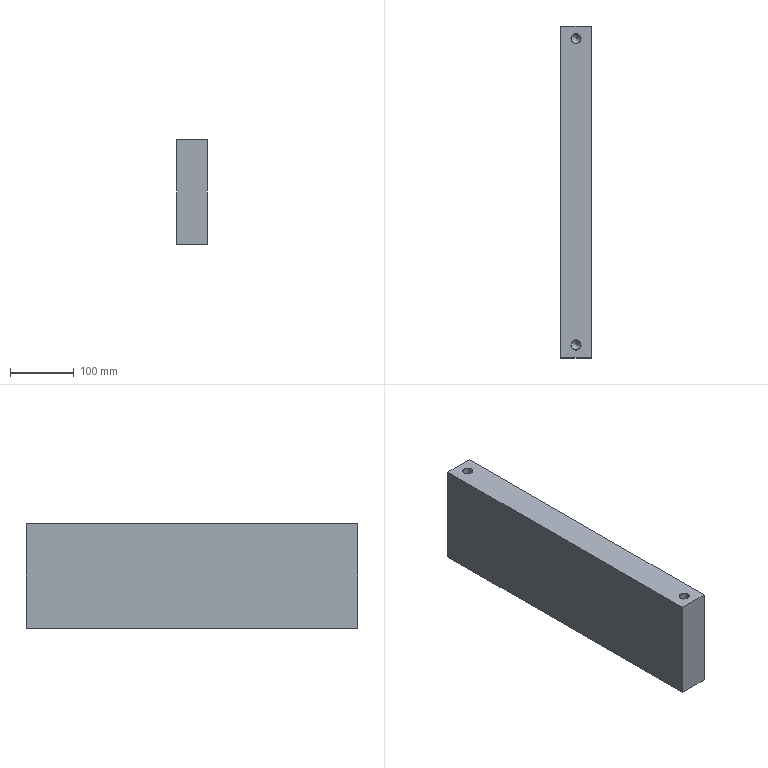Part | NX | features B2-3 2 | 1 solid | 18 faces | box 48 x 520 x 163 mm | volume 4027167 mm3 | cone 8 | plane 6 | cylinder 4 | commonest cylinder face diameters 14.506 x4
STEP:
#1=CARTESIAN_POINT('',(3450.094,-599.122,733.716));
#2=VERTEX_POINT('',#1);
#3=CARTESIAN_POINT('',(3450.094,-1119.122,733.716));
#4=VERTEX_POINT('',#3);
#5=CARTESIAN_POINT('',(3450.094,-599.122,733.716));
#6=DIRECTION('',(0.,-1.,0.));
#7=VECTOR('',#6,1000.);
#8=LINE('',#5,#7);
#9=EDGE_CURVE('',#2,#4,#8,.T.);
#10=ORIENTED_EDGE('',*,*,#9,.T.);
#11=CARTESIAN_POINT('',(3450.094,-1119.122,570.716));
#12=VERTEX_POINT('',#11);
#13=CARTESIAN_POINT('',(3450.094,-1119.122,600.716));
#14=DIRECTION('',(0.,0.,1.));
#15=VECTOR('',#14,1000.);
#16=LINE('',#13,#15);
#17=EDGE_CURVE('',#12,#4,#16,.T.);
#18=ORIENTED_EDGE('',*,*,#17,.F.);
#19=CARTESIAN_POINT('',(3450.094,-599.122,570.716));
#20=VERTEX_POINT('',#19);
#21=CARTESIAN_POINT('',(3450.094,-599.122,570.716));
#22=DIRECTION('',(0.,-1.,0.));
#23=VECTOR('',#22,1000.);
#24=LINE('',#21,#23);
#25=EDGE_CURVE('',#20,#12,#24,.T.);
#26=ORIENTED_EDGE('',*,*,#25,.F.);
#27=CARTESIAN_POINT('',(3450.094,-599.122,600.716));
#28=DIRECTION('',(0.,0.,1.));
#29=VECTOR('',#28,1000.);
#30=LINE('',#27,#29);
#31=EDGE_CURVE('',#20,#2,#30,.T.);
#32=ORIENTED_EDGE('',*,*,#31,.T.);
#33=EDGE_LOOP('',(#10,#18,#26,#32));
#34=FACE_BOUND('',#33,.T.);
#35=CARTESIAN_POINT('',(3450.094,-599.122,600.716));
#36=DIRECTION('',(-1.,0.,0.));
#37=DIRECTION('',(0.,0.,1.));
#38=AXIS2_PLACEMENT_3D('',#35,#36,#37);
#39=PLANE('',#38);
#40=ADVANCED_FACE('',(#34),#39,.F.);
#41=CARTESIAN_POINT('',(3418.094,-1039.122,570.716));
#42=VERTEX_POINT('',#41);
#43=CARTESIAN_POINT('',(3426.094,-1039.122,570.716));
#44=DIRECTION('',(0.,0.,-1.));
#45=DIRECTION('',(-1.,0.,0.));
#46=AXIS2_PLACEMENT_3D('',#43,#44,#45);
#47=CIRCLE('',#46,8.);
#48=EDGE_CURVE('',#42,#42,#47,.T.);
#49=ORIENTED_EDGE('',*,*,#48,.F.);
#50=EDGE_LOOP('',(#49));
#51=FACE_BOUND('',#50,.T.);
#52=CARTESIAN_POINT('',(3418.094,-679.122,570.716));
#53=VERTEX_POINT('',#52);
#54=CARTESIAN_POINT('',(3426.094,-679.122,570.716));
#55=DIRECTION('',(0.,0.,-1.));
#56=DIRECTION('',(-1.,0.,0.));
#57=AXIS2_PLACEMENT_3D('',#54,#55,#56);
#58=CIRCLE('',#57,8.);
#59=EDGE_CURVE('',#53,#53,#58,.T.);
#60=ORIENTED_EDGE('',*,*,#59,.F.);
#61=EDGE_LOOP('',(#60));
#62=FACE_BOUND('',#61,.T.);
#63=CARTESIAN_POINT('',(3402.094,-599.122,570.716));
#64=VERTEX_POINT('',#63);
#65=CARTESIAN_POINT('',(3402.094,-1119.122,570.716));
#66=VERTEX_POINT('',#65);
#67=CARTESIAN_POINT('',(3402.094,0.,570.716));
#68=DIRECTION('',(0.,-1.,0.));
#69=VECTOR('',#68,1000.);
#70=LINE('',#67,#69);
#71=EDGE_CURVE('',#64,#66,#70,.T.);
#72=ORIENTED_EDGE('',*,*,#71,.F.);
#73=CARTESIAN_POINT('',(1325.094,-599.122,570.716));
#74=DIRECTION('',(1.,0.,0.));
#75=VECTOR('',#74,1000.);
#76=LINE('',#73,#75);
#77=EDGE_CURVE('',#64,#20,#76,.T.);
#78=ORIENTED_EDGE('',*,*,#77,.T.);
#79=ORIENTED_EDGE('',*,*,#25,.T.);
#80=CARTESIAN_POINT('',(3450.094,-1119.122,570.716));
#81=DIRECTION('',(-1.,0.,0.));
#82=VECTOR('',#81,1000.);
#83=LINE('',#80,#82);
#84=EDGE_CURVE('',#12,#66,#83,.T.);
#85=ORIENTED_EDGE('',*,*,#84,.T.);
#86=EDGE_LOOP('',(#72,#78,#79,#85));
#87=FACE_BOUND('',#86,.T.);
#88=CARTESIAN_POINT('',(-930.,0.,570.716));
#89=DIRECTION('',(0.,0.,-1.));
#90=DIRECTION('',(-1.,0.,0.));
#91=AXIS2_PLACEMENT_3D('',#88,#89,#90);
#92=PLANE('',#91);
#93=ADVANCED_FACE('',(#51,#62,#87),#92,.T.);
#94=CARTESIAN_POINT('',(3434.094,-619.122,733.716));
#95=VERTEX_POINT('',#94);
#96=CARTESIAN_POINT('',(3426.094,-619.122,733.716));
#97=DIRECTION('',(0.,0.,1.));
#98=DIRECTION('',(1.,0.,0.));
#99=AXIS2_PLACEMENT_3D('',#96,#97,#98);
#100=CIRCLE('',#99,8.);
#101=EDGE_CURVE('',#95,#95,#100,.T.);
#102=ORIENTED_EDGE('',*,*,#101,.F.);
#103=EDGE_LOOP('',(#102));
#104=FACE_BOUND('',#103,.T.);
#105=CARTESIAN_POINT('',(3434.094,-1099.122,733.716));
#106=VERTEX_POINT('',#105);
#107=CARTESIAN_POINT('',(3426.094,-1099.122,733.716));
#108=DIRECTION('',(0.,0.,1.));
#109=DIRECTION('',(1.,0.,0.));
#110=AXIS2_PLACEMENT_3D('',#107,#108,#109);
#111=CIRCLE('',#110,8.);
#112=EDGE_CURVE('',#106,#106,#111,.T.);
#113=ORIENTED_EDGE('',*,*,#112,.F.);
#114=EDGE_LOOP('',(#113));
#115=FACE_BOUND('',#114,.T.);
#116=CARTESIAN_POINT('',(3402.094,-599.122,733.716));
#117=VERTEX_POINT('',#116);
#118=CARTESIAN_POINT('',(1325.094,-599.122,733.716));
#119=DIRECTION('',(1.,0.,0.));
#120=VECTOR('',#119,1000.);
#121=LINE('',#118,#120);
#122=EDGE_CURVE('',#117,#2,#121,.T.);
#123=ORIENTED_EDGE('',*,*,#122,.F.);
#124=CARTESIAN_POINT('',(3402.094,-1119.122,733.716));
#125=VERTEX_POINT('',#124);
#126=CARTESIAN_POINT('',(3402.094,-859.122,733.716));
#127=DIRECTION('',(0.,1.,0.));
#128=VECTOR('',#127,1000.);
#129=LINE('',#126,#128);
#130=EDGE_CURVE('',#125,#117,#129,.T.);
#131=ORIENTED_EDGE('',*,*,#130,.F.);
#132=CARTESIAN_POINT('',(3450.094,-1119.122,733.716));
#133=DIRECTION('',(-1.,0.,0.));
#134=VECTOR('',#133,1000.);
#135=LINE('',#132,#134);
#136=EDGE_CURVE('',#4,#125,#135,.T.);
#137=ORIENTED_EDGE('',*,*,#136,.F.);
#138=ORIENTED_EDGE('',*,*,#9,.F.);
#139=EDGE_LOOP('',(#123,#131,#137,#138));
#140=FACE_BOUND('',#139,.T.);
#141=CARTESIAN_POINT('',(-930.,0.,733.716));
#142=DIRECTION('',(0.,0.,-1.));
#143=DIRECTION('',(-1.,0.,0.));
#144=AXIS2_PLACEMENT_3D('',#141,#142,#143);
#145=PLANE('',#144);
#146=ADVANCED_FACE('',(#104,#115,#140),#145,.F.);
#147=ORIENTED_EDGE('',*,*,#136,.T.);
#148=CARTESIAN_POINT('',(3402.094,-1119.122,600.716));
#149=DIRECTION('',(0.,0.,-1.));
#150=VECTOR('',#149,1000.);
#151=LINE('',#148,#150);
#152=EDGE_CURVE('',#125,#66,#151,.T.);
#153=ORIENTED_EDGE('',*,*,#152,.T.);
#154=ORIENTED_EDGE('',*,*,#84,.F.);
#155=ORIENTED_EDGE('',*,*,#17,.T.);
#156=EDGE_LOOP('',(#147,#153,#154,#155));
#157=FACE_BOUND('',#156,.T.);
#158=CARTESIAN_POINT('',(3450.094,-1119.122,600.716));
#159=DIRECTION('',(0.,1.,0.));
#160=DIRECTION('',(-1.,0.,0.));
#161=AXIS2_PLACEMENT_3D('',#158,#159,#160);
#162=PLANE('',#161);
#163=ADVANCED_FACE('',(#157),#162,.F.);
#164=ORIENTED_EDGE('',*,*,#77,.F.);
#165=CARTESIAN_POINT('',(3402.094,-599.122,600.716));
#166=DIRECTION('',(0.,0.,1.));
#167=VECTOR('',#166,1000.);
#168=LINE('',#165,#167);
#169=EDGE_CURVE('',#64,#117,#168,.T.);
#170=ORIENTED_EDGE('',*,*,#169,.T.);
#171=ORIENTED_EDGE('',*,*,#122,.T.);
#172=ORIENTED_EDGE('',*,*,#31,.F.);
#173=EDGE_LOOP('',(#164,#170,#171,#172));
#174=FACE_BOUND('',#173,.T.);
#175=CARTESIAN_POINT('',(1325.094,-599.122,600.716));
#176=DIRECTION('',(0.,-1.,0.));
#177=DIRECTION('',(0.,0.,-1.));
#178=AXIS2_PLACEMENT_3D('',#175,#176,#177);
#179=PLANE('',#178);
#180=ADVANCED_FACE('',(#174),#179,.F.);
#181=ORIENTED_EDGE('',*,*,#71,.T.);
#182=ORIENTED_EDGE('',*,*,#152,.F.);
#183=ORIENTED_EDGE('',*,*,#130,.T.);
#184=ORIENTED_EDGE('',*,*,#169,.F.);
#185=EDGE_LOOP('',(#181,#182,#183,#184));
#186=FACE_BOUND('',#185,.T.);
#187=CARTESIAN_POINT('',(3402.094,-859.122,667.216));
#188=DIRECTION('',(1.,0.,0.));
#189=DIRECTION('',(0.,0.,-1.));
#190=AXIS2_PLACEMENT_3D('',#187,#188,#189);
#191=PLANE('',#190);
#192=ADVANCED_FACE('',(#186),#191,.F.);
#193=CARTESIAN_POINT('',(3433.347,-1099.122,732.969));
#194=VERTEX_POINT('',#193);
#195=CARTESIAN_POINT('',(3426.094,-1099.122,732.969));
#196=DIRECTION('',(0.,0.,1.));
#197=DIRECTION('',(1.,0.,0.));
#198=AXIS2_PLACEMENT_3D('',#195,#196,#197);
#199=CIRCLE('',#198,7.253);
#200=EDGE_CURVE('',#194,#194,#199,.F.);
#201=ORIENTED_EDGE('',*,*,#200,.F.);
#202=EDGE_LOOP('',(#201));
#203=FACE_BOUND('',#202,.T.);
#204=CARTESIAN_POINT('',(3433.347,-1099.122,688.719));
#205=VERTEX_POINT('',#204);
#206=CARTESIAN_POINT('',(3426.094,-1099.122,688.719));
#207=DIRECTION('',(0.,0.,1.));
#208=DIRECTION('',(1.,0.,0.));
#209=AXIS2_PLACEMENT_3D('',#206,#207,#208);
#210=CIRCLE('',#209,7.253);
#211=EDGE_CURVE('',#205,#205,#210,.F.);
#212=ORIENTED_EDGE('',*,*,#211,.T.);
#213=EDGE_LOOP('',(#212));
#214=FACE_BOUND('',#213,.T.);
#215=CARTESIAN_POINT('',(3426.094,-1099.122,681.466));
#216=DIRECTION('',(0.,0.,1.));
#217=DIRECTION('',(1.,0.,0.));
#218=AXIS2_PLACEMENT_3D('',#215,#216,#217);
#219=CYLINDRICAL_SURFACE('',#218,7.253);
#220=ADVANCED_FACE('',(#203,#214),#219,.F.);
#221=CARTESIAN_POINT('',(3426.094,-1099.122,681.466));
#222=VERTEX_POINT('',#221);
#223=VERTEX_LOOP('',#222);
#224=FACE_BOUND('',#223,.T.);
#225=ORIENTED_EDGE('',*,*,#211,.F.);
#226=EDGE_LOOP('',(#225));
#227=FACE_BOUND('',#226,.T.);
#228=CARTESIAN_POINT('',(3426.094,-1099.122,688.716));
#229=DIRECTION('',(0.,0.,1.));
#230=DIRECTION('',(1.,0.,0.));
#231=AXIS2_PLACEMENT_3D('',#228,#229,#230);
#232=CONICAL_SURFACE('',#231,7.25,0.7854);
#233=ADVANCED_FACE('',(#224,#227),#232,.F.);
#234=ORIENTED_EDGE('',*,*,#200,.T.);
#235=EDGE_LOOP('',(#234));
#236=FACE_BOUND('',#235,.T.);
#237=ORIENTED_EDGE('',*,*,#112,.T.);
#238=EDGE_LOOP('',(#237));
#239=FACE_BOUND('',#238,.T.);
#240=CARTESIAN_POINT('',(3426.094,-1099.122,733.716));
#241=DIRECTION('',(0.,0.,1.));
#242=DIRECTION('',(1.,0.,0.));
#243=AXIS2_PLACEMENT_3D('',#240,#241,#242);
#244=CONICAL_SURFACE('',#243,8.,0.7854);
#245=ADVANCED_FACE('',(#236,#239),#244,.F.);
#246=CARTESIAN_POINT('',(3433.347,-619.122,732.969));
#247=VERTEX_POINT('',#246);
#248=CARTESIAN_POINT('',(3426.094,-619.122,732.969));
#249=DIRECTION('',(0.,0.,1.));
#250=DIRECTION('',(1.,0.,0.));
#251=AXIS2_PLACEMENT_3D('',#248,#249,#250);
#252=CIRCLE('',#251,7.253);
#253=EDGE_CURVE('',#247,#247,#252,.F.);
#254=ORIENTED_EDGE('',*,*,#253,.F.);
#255=EDGE_LOOP('',(#254));
#256=FACE_BOUND('',#255,.T.);
#257=CARTESIAN_POINT('',(3433.347,-619.122,688.719));
#258=VERTEX_POINT('',#257);
#259=CARTESIAN_POINT('',(3426.094,-619.122,688.719));
#260=DIRECTION('',(0.,0.,1.));
#261=DIRECTION('',(1.,0.,0.));
#262=AXIS2_PLACEMENT_3D('',#259,#260,#261);
#263=CIRCLE('',#262,7.253);
#264=EDGE_CURVE('',#258,#258,#263,.F.);
#265=ORIENTED_EDGE('',*,*,#264,.T.);
#266=EDGE_LOOP('',(#265));
#267=FACE_BOUND('',#266,.T.);
#268=CARTESIAN_POINT('',(3426.094,-619.122,681.466));
#269=DIRECTION('',(0.,0.,1.));
#270=DIRECTION('',(1.,0.,0.));
#271=AXIS2_PLACEMENT_3D('',#268,#269,#270);
#272=CYLINDRICAL_SURFACE('',#271,7.253);
#273=ADVANCED_FACE('',(#256,#267),#272,.F.);
#274=CARTESIAN_POINT('',(3426.094,-619.122,681.466));
#275=VERTEX_POINT('',#274);
#276=VERTEX_LOOP('',#275);
#277=FACE_BOUND('',#276,.T.);
#278=ORIENTED_EDGE('',*,*,#264,.F.);
#279=EDGE_LOOP('',(#278));
#280=FACE_BOUND('',#279,.T.);
#281=CARTESIAN_POINT('',(3426.094,-619.122,688.716));
#282=DIRECTION('',(0.,0.,1.));
#283=DIRECTION('',(1.,0.,0.));
#284=AXIS2_PLACEMENT_3D('',#281,#282,#283);
#285=CONICAL_SURFACE('',#284,7.25,0.7854);
#286=ADVANCED_FACE('',(#277,#280),#285,.F.);
#287=ORIENTED_EDGE('',*,*,#253,.T.);
#288=EDGE_LOOP('',(#287));
#289=FACE_BOUND('',#288,.T.);
#290=ORIENTED_EDGE('',*,*,#101,.T.);
#291=EDGE_LOOP('',(#290));
#292=FACE_BOUND('',#291,.T.);
#293=CARTESIAN_POINT('',(3426.094,-619.122,733.716));
#294=DIRECTION('',(0.,0.,1.));
#295=DIRECTION('',(1.,0.,0.));
#296=AXIS2_PLACEMENT_3D('',#293,#294,#295);
#297=CONICAL_SURFACE('',#296,8.,0.7854);
#298=ADVANCED_FACE('',(#289,#292),#297,.F.);
#299=CARTESIAN_POINT('',(3418.841,-679.122,571.463));
#300=VERTEX_POINT('',#299);
#301=CARTESIAN_POINT('',(3426.094,-679.122,571.463));
#302=DIRECTION('',(0.,0.,-1.));
#303=DIRECTION('',(-1.,0.,0.));
#304=AXIS2_PLACEMENT_3D('',#301,#302,#303);
#305=CIRCLE('',#304,7.253);
#306=EDGE_CURVE('',#300,#300,#305,.F.);
#307=ORIENTED_EDGE('',*,*,#306,.F.);
#308=EDGE_LOOP('',(#307));
#309=FACE_BOUND('',#308,.T.);
#310=CARTESIAN_POINT('',(3418.841,-679.122,645.713));
#311=VERTEX_POINT('',#310);
#312=CARTESIAN_POINT('',(3426.094,-679.122,645.713));
#313=DIRECTION('',(0.,0.,-1.));
#314=DIRECTION('',(-1.,0.,0.));
#315=AXIS2_PLACEMENT_3D('',#312,#313,#314);
#316=CIRCLE('',#315,7.253);
#317=EDGE_CURVE('',#311,#311,#316,.F.);
#318=ORIENTED_EDGE('',*,*,#317,.T.);
#319=EDGE_LOOP('',(#318));
#320=FACE_BOUND('',#319,.T.);
#321=CARTESIAN_POINT('',(3426.094,-679.122,652.966));
#322=DIRECTION('',(0.,0.,-1.));
#323=DIRECTION('',(-1.,0.,0.));
#324=AXIS2_PLACEMENT_3D('',#321,#322,#323);
#325=CYLINDRICAL_SURFACE('',#324,7.253);
#326=ADVANCED_FACE('',(#309,#320),#325,.F.);
#327=CARTESIAN_POINT('',(3426.094,-679.122,652.966));
#328=VERTEX_POINT('',#327);
#329=VERTEX_LOOP('',#328);
#330=FACE_BOUND('',#329,.T.);
#331=ORIENTED_EDGE('',*,*,#317,.F.);
#332=EDGE_LOOP('',(#331));
#333=FACE_BOUND('',#332,.T.);
#334=CARTESIAN_POINT('',(3426.094,-679.122,645.716));
#335=DIRECTION('',(0.,0.,-1.));
#336=DIRECTION('',(-1.,0.,0.));
#337=AXIS2_PLACEMENT_3D('',#334,#335,#336);
#338=CONICAL_SURFACE('',#337,7.25,0.7854);
#339=ADVANCED_FACE('',(#330,#333),#338,.F.);
#340=ORIENTED_EDGE('',*,*,#306,.T.);
#341=EDGE_LOOP('',(#340));
#342=FACE_BOUND('',#341,.T.);
#343=ORIENTED_EDGE('',*,*,#59,.T.);
#344=EDGE_LOOP('',(#343));
#345=FACE_BOUND('',#344,.T.);
#346=CARTESIAN_POINT('',(3426.094,-679.122,570.716));
#347=DIRECTION('',(0.,0.,-1.));
#348=DIRECTION('',(-1.,0.,0.));
#349=AXIS2_PLACEMENT_3D('',#346,#347,#348);
#350=CONICAL_SURFACE('',#349,8.,0.7854);
#351=ADVANCED_FACE('',(#342,#345),#350,.F.);
#352=CARTESIAN_POINT('',(3418.841,-1039.122,571.463));
#353=VERTEX_POINT('',#352);
#354=CARTESIAN_POINT('',(3426.094,-1039.122,571.463));
#355=DIRECTION('',(0.,0.,-1.));
#356=DIRECTION('',(-1.,0.,0.));
#357=AXIS2_PLACEMENT_3D('',#354,#355,#356);
#358=CIRCLE('',#357,7.253);
#359=EDGE_CURVE('',#353,#353,#358,.F.);
#360=ORIENTED_EDGE('',*,*,#359,.F.);
#361=EDGE_LOOP('',(#360));
#362=FACE_BOUND('',#361,.T.);
#363=CARTESIAN_POINT('',(3418.841,-1039.122,645.713));
#364=VERTEX_POINT('',#363);
#365=CARTESIAN_POINT('',(3426.094,-1039.122,645.713));
#366=DIRECTION('',(0.,0.,-1.));
#367=DIRECTION('',(-1.,0.,0.));
#368=AXIS2_PLACEMENT_3D('',#365,#366,#367);
#369=CIRCLE('',#368,7.253);
#370=EDGE_CURVE('',#364,#364,#369,.F.);
#371=ORIENTED_EDGE('',*,*,#370,.T.);
#372=EDGE_LOOP('',(#371));
#373=FACE_BOUND('',#372,.T.);
#374=CARTESIAN_POINT('',(3426.094,-1039.122,652.966));
#375=DIRECTION('',(0.,0.,-1.));
#376=DIRECTION('',(-1.,0.,0.));
#377=AXIS2_PLACEMENT_3D('',#374,#375,#376);
#378=CYLINDRICAL_SURFACE('',#377,7.253);
#379=ADVANCED_FACE('',(#362,#373),#378,.F.);
#380=CARTESIAN_POINT('',(3426.094,-1039.122,652.966));
#381=VERTEX_POINT('',#380);
#382=VERTEX_LOOP('',#381);
#383=FACE_BOUND('',#382,.T.);
#384=ORIENTED_EDGE('',*,*,#370,.F.);
#385=EDGE_LOOP('',(#384));
#386=FACE_BOUND('',#385,.T.);
#387=CARTESIAN_POINT('',(3426.094,-1039.122,645.716));
#388=DIRECTION('',(0.,0.,-1.));
#389=DIRECTION('',(-1.,0.,0.));
#390=AXIS2_PLACEMENT_3D('',#387,#388,#389);
#391=CONICAL_SURFACE('',#390,7.25,0.7854);
#392=ADVANCED_FACE('',(#383,#386),#391,.F.);
#393=ORIENTED_EDGE('',*,*,#359,.T.);
#394=EDGE_LOOP('',(#393));
#395=FACE_BOUND('',#394,.T.);
#396=ORIENTED_EDGE('',*,*,#48,.T.);
#397=EDGE_LOOP('',(#396));
#398=FACE_BOUND('',#397,.T.);
#399=CARTESIAN_POINT('',(3426.094,-1039.122,570.716));
#400=DIRECTION('',(0.,0.,-1.));
#401=DIRECTION('',(-1.,0.,0.));
#402=AXIS2_PLACEMENT_3D('',#399,#400,#401);
#403=CONICAL_SURFACE('',#402,8.,0.7854);
#404=ADVANCED_FACE('',(#395,#398),#403,.F.);
#405=CLOSED_SHELL('',(#40,#93,#146,#163,#180,#192,#220,#233,#245,#273,#286,#298,#326,#339,#351,#379,#392,#404));
#406=MANIFOLD_SOLID_BREP('',#405);
#407=(LENGTH_UNIT()NAMED_UNIT(*)SI_UNIT(.MILLI.,.METRE.));
#408=UNCERTAINTY_MEASURE_WITH_UNIT(LENGTH_MEASURE(0.00001),#407,'','');
#409=(NAMED_UNIT(*)PLANE_ANGLE_UNIT()SI_UNIT($,.RADIAN.));
#410=(NAMED_UNIT(*)SI_UNIT($,.STERADIAN.)SOLID_ANGLE_UNIT());
#411=(GEOMETRIC_REPRESENTATION_CONTEXT(3)GLOBAL_UNCERTAINTY_ASSIGNED_CONTEXT((#408))GLOBAL_UNIT_ASSIGNED_CONTEXT((#407,#409,#410))REPRESENTATION_CONTEXT('',''));
#412=ADVANCED_BREP_SHAPE_REPRESENTATION('',(#406),#411);